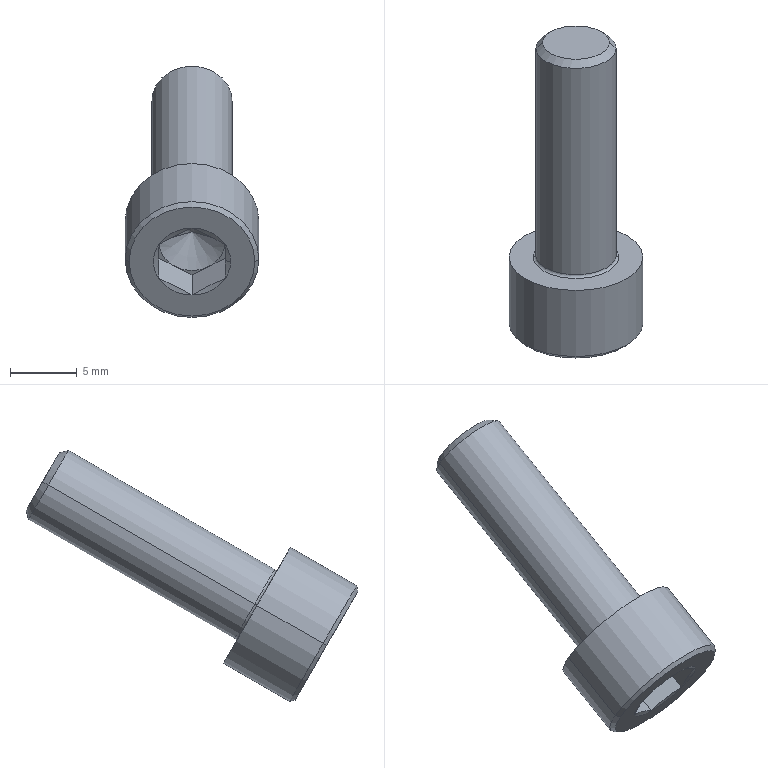Part | SolidWorks | features BaseBody 1 | 1 solid | 34 faces | box 10 x 24.818 x 18.778 mm | volume 916.28 mm3 | plane 15 | cone 13 | cylinder 4 | torus 2 | commonest cylinder face diameters 6 x2 10 x2
STEP:
#1=CARTESIAN_POINT('',(133.,-39.453,-22.778));
#2=VERTEX_POINT('',#1);
#3=CARTESIAN_POINT('',(135.5,-40.703,-23.5));
#4=VERTEX_POINT('',#3);
#5=CARTESIAN_POINT('',(135.5,-40.703,-23.5));
#6=DIRECTION('',(0.866,-0.433,-0.25));
#7=VECTOR('',#6,1000.);
#8=LINE('',#5,#7);
#9=EDGE_CURVE('',#2,#4,#8,.T.);
#10=ORIENTED_EDGE('',*,*,#9,.F.);
#11=CARTESIAN_POINT('',(130.5,-40.703,-23.5));
#12=VERTEX_POINT('',#11);
#13=CARTESIAN_POINT('',(130.5,-40.703,-23.5));
#14=DIRECTION('',(-0.866,-0.433,-0.25));
#15=VECTOR('',#14,1000.);
#16=LINE('',#13,#15);
#17=EDGE_CURVE('',#2,#12,#16,.T.);
#18=ORIENTED_EDGE('',*,*,#17,.T.);
#19=CARTESIAN_POINT('',(131.75,-39.621,-25.375));
#20=VERTEX_POINT('',#19);
#21=CARTESIAN_POINT('',(133.,-40.703,-23.5));
#22=DIRECTION('',(0.,-0.866,-0.5));
#23=DIRECTION('',(1.,0.,0.));
#24=AXIS2_PLACEMENT_3D('',#21,#22,#23);
#25=CIRCLE('',#24,2.5);
#26=EDGE_CURVE('',#12,#20,#25,.T.);
#27=ORIENTED_EDGE('',*,*,#26,.T.);
#28=CARTESIAN_POINT('',(134.25,-39.621,-25.375));
#29=VERTEX_POINT('',#28);
#30=CARTESIAN_POINT('',(133.,-40.703,-23.5));
#31=DIRECTION('',(0.,-0.866,-0.5));
#32=DIRECTION('',(1.,0.,0.));
#33=AXIS2_PLACEMENT_3D('',#30,#31,#32);
#34=CIRCLE('',#33,2.5);
#35=EDGE_CURVE('',#20,#29,#34,.T.);
#36=ORIENTED_EDGE('',*,*,#35,.T.);
#37=CARTESIAN_POINT('',(133.,-40.703,-23.5));
#38=DIRECTION('',(0.,-0.866,-0.5));
#39=DIRECTION('',(1.,0.,0.));
#40=AXIS2_PLACEMENT_3D('',#37,#38,#39);
#41=CIRCLE('',#40,2.5);
#42=EDGE_CURVE('',#29,#4,#41,.T.);
#43=ORIENTED_EDGE('',*,*,#42,.T.);
#44=EDGE_LOOP('',(#10,#18,#27,#36,#43));
#45=FACE_OUTER_BOUND('',#44,.T.);
#46=CARTESIAN_POINT('',(133.,-40.703,-23.5));
#47=DIRECTION('',(0.,-0.866,-0.5));
#48=DIRECTION('',(1.,0.,0.));
#49=AXIS2_PLACEMENT_3D('',#46,#47,#48);
#50=CONICAL_SURFACE('',#49,2.5,1.047);
#51=ADVANCED_FACE('',(#45),#50,.F.);
#52=CARTESIAN_POINT('',(135.5,-43.212,-24.948));
#53=VERTEX_POINT('',#52);
#54=CARTESIAN_POINT('',(135.5,-44.023,-23.75));
#55=VERTEX_POINT('',#54);
#56=CARTESIAN_POINT('',(135.5,-43.212,-24.948));
#57=CARTESIAN_POINT('',(135.5,-43.453,-24.531));
#58=CARTESIAN_POINT('',(135.5,-43.727,-24.134));
#59=CARTESIAN_POINT('',(135.5,-44.023,-23.75));
#60=B_SPLINE_CURVE_WITH_KNOTS('',3,(#56,#57,#58,#59),.UNSPECIFIED.,.F.,.F.,(4,4),(0.003815,0.005271),.UNSPECIFIED.);
#61=EDGE_CURVE('',#53,#55,#60,.T.);
#62=ORIENTED_EDGE('',*,*,#61,.F.);
#63=CARTESIAN_POINT('',(135.887,-43.301,-25.));
#64=VERTEX_POINT('',#63);
#65=CARTESIAN_POINT('',(135.887,-43.301,-25.));
#66=DIRECTION('',(0.9659,-0.2241,-0.1294));
#67=VECTOR('',#66,1000.);
#68=LINE('',#65,#67);
#69=EDGE_CURVE('',#53,#64,#68,.T.);
#70=ORIENTED_EDGE('',*,*,#69,.T.);
#71=CARTESIAN_POINT('',(133.,-43.301,-25.));
#72=DIRECTION('',(0.,-0.866,-0.5));
#73=DIRECTION('',(1.,0.,0.));
#74=AXIS2_PLACEMENT_3D('',#71,#72,#73);
#75=CIRCLE('',#74,2.887);
#76=EDGE_CURVE('',#64,#55,#75,.T.);
#77=ORIENTED_EDGE('',*,*,#76,.T.);
#78=EDGE_LOOP('',(#62,#70,#77));
#79=FACE_OUTER_BOUND('',#78,.T.);
#80=CARTESIAN_POINT('',(133.,-43.301,-25.));
#81=DIRECTION('',(0.,-0.866,-0.5));
#82=DIRECTION('',(1.,0.,0.));
#83=AXIS2_PLACEMENT_3D('',#80,#81,#82);
#84=CONICAL_SURFACE('',#83,2.887,1.309);
#85=ADVANCED_FACE('',(#79),#84,.F.);
#86=CARTESIAN_POINT('',(130.5,-22.084,-12.75));
#87=VERTEX_POINT('',#86);
#88=CARTESIAN_POINT('',(135.5,-22.084,-12.75));
#89=VERTEX_POINT('',#88);
#90=CARTESIAN_POINT('',(133.,-22.084,-12.75));
#91=DIRECTION('',(0.,0.866,0.5));
#92=DIRECTION('',(-1.,0.,0.));
#93=AXIS2_PLACEMENT_3D('',#90,#91,#92);
#94=CIRCLE('',#93,2.5);
#95=EDGE_CURVE('',#87,#89,#94,.T.);
#96=ORIENTED_EDGE('',*,*,#95,.F.);
#97=CARTESIAN_POINT('',(130.,-22.517,-13.));
#98=VERTEX_POINT('',#97);
#99=CARTESIAN_POINT('',(130.5,-22.084,-12.75));
#100=DIRECTION('',(-0.7071,-0.6124,-0.3536));
#101=VECTOR('',#100,1000.);
#102=LINE('',#99,#101);
#103=EDGE_CURVE('',#87,#98,#102,.T.);
#104=ORIENTED_EDGE('',*,*,#103,.T.);
#105=CARTESIAN_POINT('',(136.,-22.517,-13.));
#106=VERTEX_POINT('',#105);
#107=CARTESIAN_POINT('',(133.,-22.517,-13.));
#108=DIRECTION('',(0.,-0.866,-0.5));
#109=DIRECTION('',(-1.,0.,0.));
#110=AXIS2_PLACEMENT_3D('',#107,#108,#109);
#111=CIRCLE('',#110,3.);
#112=EDGE_CURVE('',#106,#98,#111,.T.);
#113=ORIENTED_EDGE('',*,*,#112,.F.);
#114=CARTESIAN_POINT('',(135.5,-22.084,-12.75));
#115=DIRECTION('',(0.7071,-0.6124,-0.3536));
#116=VECTOR('',#115,1000.);
#117=LINE('',#114,#116);
#118=EDGE_CURVE('',#89,#106,#117,.T.);
#119=ORIENTED_EDGE('',*,*,#118,.F.);
#120=EDGE_LOOP('',(#96,#104,#113,#119));
#121=FACE_OUTER_BOUND('',#120,.T.);
#122=CARTESIAN_POINT('',(133.,-22.084,-12.75));
#123=DIRECTION('',(0.,-0.866,-0.5));
#124=DIRECTION('',(1.,0.,0.));
#125=AXIS2_PLACEMENT_3D('',#122,#123,#124);
#126=CONICAL_SURFACE('',#125,2.5,0.7854);
#127=ADVANCED_FACE('',(#121),#126,.T.);
#128=CARTESIAN_POINT('',(136.,-37.932,-21.9));
#129=VERTEX_POINT('',#128);
#130=CARTESIAN_POINT('',(130.,-37.932,-21.9));
#131=VERTEX_POINT('',#130);
#132=CARTESIAN_POINT('',(133.,-37.932,-21.9));
#133=DIRECTION('',(0.,0.866,0.5));
#134=DIRECTION('',(-1.,0.,0.));
#135=AXIS2_PLACEMENT_3D('',#132,#133,#134);
#136=CIRCLE('',#135,3.);
#137=EDGE_CURVE('',#129,#131,#136,.T.);
#138=ORIENTED_EDGE('',*,*,#137,.F.);
#139=CARTESIAN_POINT('',(136.2,-38.105,-22.));
#140=VERTEX_POINT('',#139);
#141=CARTESIAN_POINT('',(136.2,-37.932,-21.9));
#142=DIRECTION('',(0.,-0.5,0.866));
#143=DIRECTION('',(0.,-0.866,-0.5));
#144=AXIS2_PLACEMENT_3D('',#141,#142,#143);
#145=CIRCLE('',#144,0.2);
#146=EDGE_CURVE('',#129,#140,#145,.T.);
#147=ORIENTED_EDGE('',*,*,#146,.T.);
#148=CARTESIAN_POINT('',(129.8,-38.105,-22.));
#149=VERTEX_POINT('',#148);
#150=CARTESIAN_POINT('',(133.,-38.105,-22.));
#151=DIRECTION('',(0.,-0.866,-0.5));
#152=DIRECTION('',(-1.,0.,0.));
#153=AXIS2_PLACEMENT_3D('',#150,#151,#152);
#154=CIRCLE('',#153,3.2);
#155=EDGE_CURVE('',#149,#140,#154,.T.);
#156=ORIENTED_EDGE('',*,*,#155,.F.);
#157=CARTESIAN_POINT('',(129.8,-37.932,-21.9));
#158=DIRECTION('',(0.,0.5,-0.866));
#159=DIRECTION('',(0.,0.866,0.5));
#160=AXIS2_PLACEMENT_3D('',#157,#158,#159);
#161=CIRCLE('',#160,0.2);
#162=EDGE_CURVE('',#131,#149,#161,.T.);
#163=ORIENTED_EDGE('',*,*,#162,.F.);
#164=EDGE_LOOP('',(#138,#147,#156,#163));
#165=FACE_OUTER_BOUND('',#164,.T.);
#166=CARTESIAN_POINT('',(133.,-37.932,-21.9));
#167=DIRECTION('',(0.,0.866,0.5));
#168=DIRECTION('',(-1.,0.,0.));
#169=AXIS2_PLACEMENT_3D('',#166,#167,#168);
#170=TOROIDAL_SURFACE('',#169,3.2,0.2);
#171=ADVANCED_FACE('',(#165),#170,.F.);
#172=ORIENTED_EDGE('',*,*,#112,.T.);
#173=CARTESIAN_POINT('',(130.,-22.084,-12.75));
#174=DIRECTION('',(0.,-0.866,-0.5));
#175=VECTOR('',#174,1000.);
#176=LINE('',#173,#175);
#177=EDGE_CURVE('',#98,#131,#176,.T.);
#178=ORIENTED_EDGE('',*,*,#177,.T.);
#179=CARTESIAN_POINT('',(133.,-37.932,-21.9));
#180=DIRECTION('',(0.,0.866,0.5));
#181=DIRECTION('',(-1.,0.,0.));
#182=AXIS2_PLACEMENT_3D('',#179,#180,#181);
#183=CIRCLE('',#182,3.);
#184=EDGE_CURVE('',#131,#129,#183,.T.);
#185=ORIENTED_EDGE('',*,*,#184,.T.);
#186=CARTESIAN_POINT('',(136.,-22.084,-12.75));
#187=DIRECTION('',(0.,-0.866,-0.5));
#188=VECTOR('',#187,1000.);
#189=LINE('',#186,#188);
#190=EDGE_CURVE('',#106,#129,#189,.T.);
#191=ORIENTED_EDGE('',*,*,#190,.F.);
#192=EDGE_LOOP('',(#172,#178,#185,#191));
#193=FACE_OUTER_BOUND('',#192,.T.);
#194=CARTESIAN_POINT('',(133.,-22.084,-12.75));
#195=DIRECTION('',(0.,-0.866,-0.5));
#196=DIRECTION('',(1.,0.,0.));
#197=AXIS2_PLACEMENT_3D('',#194,#195,#196);
#198=CYLINDRICAL_SURFACE('',#197,3.);
#199=ADVANCED_FACE('',(#193),#198,.T.);
#200=CARTESIAN_POINT('',(137.7,-43.301,-25.));
#201=VERTEX_POINT('',#200);
#202=CARTESIAN_POINT('',(128.3,-43.301,-25.));
#203=VERTEX_POINT('',#202);
#204=CARTESIAN_POINT('',(133.,-43.301,-25.));
#205=DIRECTION('',(0.,-0.866,-0.5));
#206=DIRECTION('',(-1.,0.,0.));
#207=AXIS2_PLACEMENT_3D('',#204,#205,#206);
#208=CIRCLE('',#207,4.7);
#209=EDGE_CURVE('',#201,#203,#208,.T.);
#210=ORIENTED_EDGE('',*,*,#209,.F.);
#211=CARTESIAN_POINT('',(138.,-43.041,-24.85));
#212=VERTEX_POINT('',#211);
#213=CARTESIAN_POINT('',(138.,-43.041,-24.85));
#214=DIRECTION('',(0.7071,0.6124,0.3536));
#215=VECTOR('',#214,1000.);
#216=LINE('',#213,#215);
#217=EDGE_CURVE('',#201,#212,#216,.T.);
#218=ORIENTED_EDGE('',*,*,#217,.T.);
#219=CARTESIAN_POINT('',(128.,-43.041,-24.85));
#220=VERTEX_POINT('',#219);
#221=CARTESIAN_POINT('',(133.,-43.041,-24.85));
#222=DIRECTION('',(0.,0.866,0.5));
#223=DIRECTION('',(-1.,0.,0.));
#224=AXIS2_PLACEMENT_3D('',#221,#222,#223);
#225=CIRCLE('',#224,5.);
#226=EDGE_CURVE('',#220,#212,#225,.T.);
#227=ORIENTED_EDGE('',*,*,#226,.F.);
#228=CARTESIAN_POINT('',(128.,-43.041,-24.85));
#229=DIRECTION('',(-0.7071,0.6124,0.3536));
#230=VECTOR('',#229,1000.);
#231=LINE('',#228,#230);
#232=EDGE_CURVE('',#203,#220,#231,.T.);
#233=ORIENTED_EDGE('',*,*,#232,.F.);
#234=EDGE_LOOP('',(#210,#218,#227,#233));
#235=FACE_OUTER_BOUND('',#234,.T.);
#236=CARTESIAN_POINT('',(133.,-43.041,-24.85));
#237=DIRECTION('',(0.,0.866,0.5));
#238=DIRECTION('',(-1.,0.,0.));
#239=AXIS2_PLACEMENT_3D('',#236,#237,#238);
#240=CONICAL_SURFACE('',#239,5.,0.7854);
#241=ADVANCED_FACE('',(#235),#240,.T.);
#242=CARTESIAN_POINT('',(128.,-38.105,-22.));
#243=VERTEX_POINT('',#242);
#244=CARTESIAN_POINT('',(138.,-38.105,-22.));
#245=VERTEX_POINT('',#244);
#246=CARTESIAN_POINT('',(133.,-38.105,-22.));
#247=DIRECTION('',(0.,0.866,0.5));
#248=DIRECTION('',(-1.,0.,0.));
#249=AXIS2_PLACEMENT_3D('',#246,#247,#248);
#250=CIRCLE('',#249,5.);
#251=EDGE_CURVE('',#243,#245,#250,.T.);
#252=ORIENTED_EDGE('',*,*,#251,.F.);
#253=CARTESIAN_POINT('',(128.,-38.105,-22.));
#254=DIRECTION('',(0.,-0.866,-0.5));
#255=VECTOR('',#254,1000.);
#256=LINE('',#253,#255);
#257=EDGE_CURVE('',#243,#220,#256,.T.);
#258=ORIENTED_EDGE('',*,*,#257,.T.);
#259=ORIENTED_EDGE('',*,*,#226,.T.);
#260=CARTESIAN_POINT('',(138.,-38.105,-22.));
#261=DIRECTION('',(0.,-0.866,-0.5));
#262=VECTOR('',#261,1000.);
#263=LINE('',#260,#262);
#264=EDGE_CURVE('',#245,#212,#263,.T.);
#265=ORIENTED_EDGE('',*,*,#264,.F.);
#266=EDGE_LOOP('',(#252,#258,#259,#265));
#267=FACE_OUTER_BOUND('',#266,.T.);
#268=CARTESIAN_POINT('',(133.,-38.105,-22.));
#269=DIRECTION('',(0.,-0.866,-0.5));
#270=DIRECTION('',(1.,0.,0.));
#271=AXIS2_PLACEMENT_3D('',#268,#269,#270);
#272=CYLINDRICAL_SURFACE('',#271,5.);
#273=ADVANCED_FACE('',(#267),#272,.T.);
#274=ORIENTED_EDGE('',*,*,#155,.T.);
#275=CARTESIAN_POINT('',(133.,-38.105,-22.));
#276=DIRECTION('',(0.,-0.866,-0.5));
#277=DIRECTION('',(-1.,0.,0.));
#278=AXIS2_PLACEMENT_3D('',#275,#276,#277);
#279=CIRCLE('',#278,3.2);
#280=EDGE_CURVE('',#140,#149,#279,.T.);
#281=ORIENTED_EDGE('',*,*,#280,.T.);
#282=EDGE_LOOP('',(#274,#281));
#283=FACE_BOUND('',#282,.T.);
#284=CARTESIAN_POINT('',(133.,-38.105,-22.));
#285=DIRECTION('',(0.,0.866,0.5));
#286=DIRECTION('',(-1.,0.,0.));
#287=AXIS2_PLACEMENT_3D('',#284,#285,#286);
#288=CIRCLE('',#287,5.);
#289=EDGE_CURVE('',#245,#243,#288,.T.);
#290=ORIENTED_EDGE('',*,*,#289,.T.);
#291=ORIENTED_EDGE('',*,*,#251,.T.);
#292=EDGE_LOOP('',(#290,#291));
#293=FACE_OUTER_BOUND('',#292,.T.);
#294=CARTESIAN_POINT('',(133.,-38.105,-22.));
#295=DIRECTION('',(0.,0.866,0.5));
#296=DIRECTION('',(-1.,0.,0.));
#297=AXIS2_PLACEMENT_3D('',#294,#295,#296);
#298=PLANE('',#297);
#299=ADVANCED_FACE('',(#283,#293),#298,.T.);
#300=ORIENTED_EDGE('',*,*,#257,.F.);
#301=ORIENTED_EDGE('',*,*,#289,.F.);
#302=ORIENTED_EDGE('',*,*,#264,.T.);
#303=CARTESIAN_POINT('',(133.,-43.041,-24.85));
#304=DIRECTION('',(0.,0.866,0.5));
#305=DIRECTION('',(-1.,0.,0.));
#306=AXIS2_PLACEMENT_3D('',#303,#304,#305);
#307=CIRCLE('',#306,5.);
#308=EDGE_CURVE('',#212,#220,#307,.T.);
#309=ORIENTED_EDGE('',*,*,#308,.T.);
#310=EDGE_LOOP('',(#300,#301,#302,#309));
#311=FACE_OUTER_BOUND('',#310,.T.);
#312=CARTESIAN_POINT('',(133.,-38.105,-22.));
#313=DIRECTION('',(0.,-0.866,-0.5));
#314=DIRECTION('',(1.,0.,0.));
#315=AXIS2_PLACEMENT_3D('',#312,#313,#314);
#316=CYLINDRICAL_SURFACE('',#315,5.);
#317=ADVANCED_FACE('',(#311),#316,.T.);
#318=CARTESIAN_POINT('',(130.5,-44.023,-23.75));
#319=VERTEX_POINT('',#318);
#320=CARTESIAN_POINT('',(130.5,-42.58,-26.25));
#321=VERTEX_POINT('',#320);
#322=CARTESIAN_POINT('',(133.,-43.301,-25.));
#323=DIRECTION('',(0.,-0.866,-0.5));
#324=DIRECTION('',(1.,0.,0.));
#325=AXIS2_PLACEMENT_3D('',#322,#323,#324);
#326=CIRCLE('',#325,2.887);
#327=EDGE_CURVE('',#319,#321,#326,.T.);
#328=ORIENTED_EDGE('',*,*,#327,.F.);
#329=CARTESIAN_POINT('',(133.,-44.745,-22.5));
#330=VERTEX_POINT('',#329);
#331=CARTESIAN_POINT('',(133.,-43.301,-25.));
#332=DIRECTION('',(0.,-0.866,-0.5));
#333=DIRECTION('',(1.,0.,0.));
#334=AXIS2_PLACEMENT_3D('',#331,#332,#333);
#335=CIRCLE('',#334,2.887);
#336=EDGE_CURVE('',#330,#319,#335,.T.);
#337=ORIENTED_EDGE('',*,*,#336,.F.);
#338=CARTESIAN_POINT('',(133.,-43.301,-25.));
#339=DIRECTION('',(0.,-0.866,-0.5));
#340=DIRECTION('',(1.,0.,0.));
#341=AXIS2_PLACEMENT_3D('',#338,#339,#340);
#342=CIRCLE('',#341,2.887);
#343=EDGE_CURVE('',#55,#330,#342,.T.);
#344=ORIENTED_EDGE('',*,*,#343,.F.);
#345=ORIENTED_EDGE('',*,*,#76,.F.);
#346=CARTESIAN_POINT('',(135.5,-42.58,-26.25));
#347=VERTEX_POINT('',#346);
#348=CARTESIAN_POINT('',(133.,-43.301,-25.));
#349=DIRECTION('',(0.,-0.866,-0.5));
#350=DIRECTION('',(1.,0.,0.));
#351=AXIS2_PLACEMENT_3D('',#348,#349,#350);
#352=CIRCLE('',#351,2.887);
#353=EDGE_CURVE('',#347,#64,#352,.T.);
#354=ORIENTED_EDGE('',*,*,#353,.F.);
#355=CARTESIAN_POINT('',(133.,-41.858,-27.5));
#356=VERTEX_POINT('',#355);
#357=CARTESIAN_POINT('',(133.,-43.301,-25.));
#358=DIRECTION('',(0.,-0.866,-0.5));
#359=DIRECTION('',(1.,0.,0.));
#360=AXIS2_PLACEMENT_3D('',#357,#358,#359);
#361=CIRCLE('',#360,2.887);
#362=EDGE_CURVE('',#356,#347,#361,.T.);
#363=ORIENTED_EDGE('',*,*,#362,.F.);
#364=CARTESIAN_POINT('',(133.,-43.301,-25.));
#365=DIRECTION('',(0.,-0.866,-0.5));
#366=DIRECTION('',(1.,0.,0.));
#367=AXIS2_PLACEMENT_3D('',#364,#365,#366);
#368=CIRCLE('',#367,2.887);
#369=EDGE_CURVE('',#321,#356,#368,.T.);
#370=ORIENTED_EDGE('',*,*,#369,.F.);
#371=EDGE_LOOP('',(#328,#337,#344,#345,#354,#363,#370));
#372=FACE_BOUND('',#371,.T.);
#373=CARTESIAN_POINT('',(133.,-43.301,-25.));
#374=DIRECTION('',(0.,-0.866,-0.5));
#375=DIRECTION('',(-1.,0.,0.));
#376=AXIS2_PLACEMENT_3D('',#373,#374,#375);
#377=CIRCLE('',#376,4.7);
#378=EDGE_CURVE('',#203,#201,#377,.T.);
#379=ORIENTED_EDGE('',*,*,#378,.T.);
#380=ORIENTED_EDGE('',*,*,#209,.T.);
#381=EDGE_LOOP('',(#379,#380));
#382=FACE_OUTER_BOUND('',#381,.T.);
#383=CARTESIAN_POINT('',(133.,-43.301,-25.));
#384=DIRECTION('',(0.,0.866,0.5));
#385=DIRECTION('',(-1.,0.,0.));
#386=AXIS2_PLACEMENT_3D('',#383,#384,#385);
#387=PLANE('',#386);
#388=ADVANCED_FACE('',(#372,#382),#387,.F.);
#389=ORIENTED_EDGE('',*,*,#217,.F.);
#390=ORIENTED_EDGE('',*,*,#378,.F.);
#391=ORIENTED_EDGE('',*,*,#232,.T.);
#392=ORIENTED_EDGE('',*,*,#308,.F.);
#393=EDGE_LOOP('',(#389,#390,#391,#392));
#394=FACE_OUTER_BOUND('',#393,.T.);
#395=CARTESIAN_POINT('',(133.,-43.041,-24.85));
#396=DIRECTION('',(0.,0.866,0.5));
#397=DIRECTION('',(-1.,0.,0.));
#398=AXIS2_PLACEMENT_3D('',#395,#396,#397);
#399=CONICAL_SURFACE('',#398,5.,0.7854);
#400=ADVANCED_FACE('',(#394),#399,.T.);
#401=ORIENTED_EDGE('',*,*,#177,.F.);
#402=CARTESIAN_POINT('',(133.,-22.517,-13.));
#403=DIRECTION('',(0.,-0.866,-0.5));
#404=DIRECTION('',(-1.,0.,0.));
#405=AXIS2_PLACEMENT_3D('',#402,#403,#404);
#406=CIRCLE('',#405,3.);
#407=EDGE_CURVE('',#98,#106,#406,.T.);
#408=ORIENTED_EDGE('',*,*,#407,.T.);
#409=ORIENTED_EDGE('',*,*,#190,.T.);
#410=ORIENTED_EDGE('',*,*,#137,.T.);
#411=EDGE_LOOP('',(#401,#408,#409,#410));
#412=FACE_OUTER_BOUND('',#411,.T.);
#413=CARTESIAN_POINT('',(133.,-22.084,-12.75));
#414=DIRECTION('',(0.,-0.866,-0.5));
#415=DIRECTION('',(1.,0.,0.));
#416=AXIS2_PLACEMENT_3D('',#413,#414,#415);
#417=CYLINDRICAL_SURFACE('',#416,3.);
#418=ADVANCED_FACE('',(#412),#417,.T.);
#419=CARTESIAN_POINT('',(133.,-22.084,-12.75));
#420=DIRECTION('',(0.,0.866,0.5));
#421=DIRECTION('',(-1.,0.,0.));
#422=AXIS2_PLACEMENT_3D('',#419,#420,#421);
#423=CIRCLE('',#422,2.5);
#424=EDGE_CURVE('',#89,#87,#423,.T.);
#425=ORIENTED_EDGE('',*,*,#424,.T.);
#426=ORIENTED_EDGE('',*,*,#95,.T.);
#427=EDGE_LOOP('',(#425,#426));
#428=FACE_OUTER_BOUND('',#427,.T.);
#429=CARTESIAN_POINT('',(133.,-22.084,-12.75));
#430=DIRECTION('',(0.,0.866,0.5));
#431=DIRECTION('',(-1.,0.,0.));
#432=AXIS2_PLACEMENT_3D('',#429,#430,#431);
#433=PLANE('',#432);
#434=ADVANCED_FACE('',(#428),#433,.T.);
#435=ORIENTED_EDGE('',*,*,#146,.F.);
#436=ORIENTED_EDGE('',*,*,#184,.F.);
#437=ORIENTED_EDGE('',*,*,#162,.T.);
#438=ORIENTED_EDGE('',*,*,#280,.F.);
#439=EDGE_LOOP('',(#435,#436,#437,#438));
#440=FACE_OUTER_BOUND('',#439,.T.);
#441=CARTESIAN_POINT('',(133.,-37.932,-21.9));
#442=DIRECTION('',(0.,0.866,0.5));
#443=DIRECTION('',(-1.,0.,0.));
#444=AXIS2_PLACEMENT_3D('',#441,#442,#443);
#445=TOROIDAL_SURFACE('',#444,3.2,0.2);
#446=ADVANCED_FACE('',(#440),#445,.F.);
#447=ORIENTED_EDGE('',*,*,#103,.F.);
#448=ORIENTED_EDGE('',*,*,#424,.F.);
#449=ORIENTED_EDGE('',*,*,#118,.T.);
#450=ORIENTED_EDGE('',*,*,#407,.F.);
#451=EDGE_LOOP('',(#447,#448,#449,#450));
#452=FACE_OUTER_BOUND('',#451,.T.);
#453=CARTESIAN_POINT('',(133.,-22.084,-12.75));
#454=DIRECTION('',(0.,-0.866,-0.5));
#455=DIRECTION('',(1.,0.,0.));
#456=AXIS2_PLACEMENT_3D('',#453,#454,#455);
#457=CONICAL_SURFACE('',#456,2.5,0.7854);
#458=ADVANCED_FACE('',(#452),#457,.T.);
#459=ORIENTED_EDGE('',*,*,#336,.T.);
#460=CARTESIAN_POINT('',(133.,-44.745,-22.5));
#461=CARTESIAN_POINT('',(132.583,-44.569,-22.676));
#462=CARTESIAN_POINT('',(131.75,-44.26,-23.054));
#463=CARTESIAN_POINT('',(130.917,-44.087,-23.509));
#464=CARTESIAN_POINT('',(130.5,-44.023,-23.75));
#465=B_SPLINE_CURVE_WITH_KNOTS('',3,(#460,#461,#462,#463,#464),.UNSPECIFIED.,.F.,.F.,(4,1,4),(0.000000231,0.001444,0.002887),.UNSPECIFIED.);
#466=EDGE_CURVE('',#330,#319,#465,.T.);
#467=ORIENTED_EDGE('',*,*,#466,.F.);
#468=EDGE_LOOP('',(#459,#467));
#469=FACE_OUTER_BOUND('',#468,.T.);
#470=CARTESIAN_POINT('',(133.,-43.301,-25.));
#471=DIRECTION('',(0.,-0.866,-0.5));
#472=DIRECTION('',(1.,0.,0.));
#473=AXIS2_PLACEMENT_3D('',#470,#471,#472);
#474=CONICAL_SURFACE('',#473,2.887,1.309);
#475=ADVANCED_FACE('',(#469),#474,.F.);
#476=ORIENTED_EDGE('',*,*,#327,.T.);
#477=CARTESIAN_POINT('',(130.5,-44.023,-23.75));
#478=CARTESIAN_POINT('',(130.5,-43.728,-24.133));
#479=CARTESIAN_POINT('',(130.5,-43.454,-24.529));
#480=CARTESIAN_POINT('',(130.5,-42.972,-25.363));
#481=CARTESIAN_POINT('',(130.5,-42.764,-25.802));
#482=CARTESIAN_POINT('',(130.5,-42.58,-26.25));
#483=B_SPLINE_CURVE_WITH_KNOTS('',3,(#477,#478,#479,#480,#481,#482),.UNSPECIFIED.,.F.,.F.,(4,2,4),(0.0002925,0.001736,0.003179),.UNSPECIFIED.);
#484=EDGE_CURVE('',#319,#321,#483,.T.);
#485=ORIENTED_EDGE('',*,*,#484,.F.);
#486=EDGE_LOOP('',(#476,#485));
#487=FACE_OUTER_BOUND('',#486,.T.);
#488=CARTESIAN_POINT('',(133.,-43.301,-25.));
#489=DIRECTION('',(0.,-0.866,-0.5));
#490=DIRECTION('',(1.,0.,0.));
#491=AXIS2_PLACEMENT_3D('',#488,#489,#490);
#492=CONICAL_SURFACE('',#491,2.887,1.309);
#493=ADVANCED_FACE('',(#487),#492,.F.);
#494=ORIENTED_EDGE('',*,*,#369,.T.);
#495=CARTESIAN_POINT('',(130.5,-42.58,-26.25));
#496=CARTESIAN_POINT('',(130.917,-42.403,-26.426));
#497=CARTESIAN_POINT('',(131.75,-42.095,-26.804));
#498=CARTESIAN_POINT('',(132.583,-41.922,-27.259));
#499=CARTESIAN_POINT('',(133.,-41.858,-27.5));
#500=B_SPLINE_CURVE_WITH_KNOTS('',3,(#495,#496,#497,#498,#499),.UNSPECIFIED.,.F.,.F.,(4,1,4),(0.000000231,0.001444,0.002887),.UNSPECIFIED.);
#501=EDGE_CURVE('',#321,#356,#500,.T.);
#502=ORIENTED_EDGE('',*,*,#501,.F.);
#503=EDGE_LOOP('',(#494,#502));
#504=FACE_OUTER_BOUND('',#503,.T.);
#505=CARTESIAN_POINT('',(133.,-43.301,-25.));
#506=DIRECTION('',(0.,-0.866,-0.5));
#507=DIRECTION('',(1.,0.,0.));
#508=AXIS2_PLACEMENT_3D('',#505,#506,#507);
#509=CONICAL_SURFACE('',#508,2.887,1.309);
#510=ADVANCED_FACE('',(#504),#509,.F.);
#511=ORIENTED_EDGE('',*,*,#362,.T.);
#512=CARTESIAN_POINT('',(133.,-41.858,-27.5));
#513=CARTESIAN_POINT('',(133.417,-41.922,-27.259));
#514=CARTESIAN_POINT('',(134.25,-42.095,-26.804));
#515=CARTESIAN_POINT('',(135.083,-42.403,-26.426));
#516=CARTESIAN_POINT('',(135.5,-42.58,-26.25));
#517=B_SPLINE_CURVE_WITH_KNOTS('',3,(#512,#513,#514,#515,#516),.UNSPECIFIED.,.F.,.F.,(4,1,4),(0.000000231,0.001444,0.002887),.UNSPECIFIED.);
#518=EDGE_CURVE('',#356,#347,#517,.T.);
#519=ORIENTED_EDGE('',*,*,#518,.F.);
#520=EDGE_LOOP('',(#511,#519));
#521=FACE_OUTER_BOUND('',#520,.T.);
#522=CARTESIAN_POINT('',(133.,-43.301,-25.));
#523=DIRECTION('',(0.,-0.866,-0.5));
#524=DIRECTION('',(1.,0.,0.));
#525=AXIS2_PLACEMENT_3D('',#522,#523,#524);
#526=CONICAL_SURFACE('',#525,2.887,1.309);
#527=ADVANCED_FACE('',(#521),#526,.F.);
#528=ORIENTED_EDGE('',*,*,#69,.F.);
#529=CARTESIAN_POINT('',(135.5,-42.58,-26.25));
#530=CARTESIAN_POINT('',(135.5,-42.764,-25.803));
#531=CARTESIAN_POINT('',(135.5,-42.971,-25.364));
#532=CARTESIAN_POINT('',(135.5,-43.212,-24.948));
#533=B_SPLINE_CURVE_WITH_KNOTS('',3,(#529,#530,#531,#532),.UNSPECIFIED.,.F.,.F.,(4,4),(0.002365,0.003815),.UNSPECIFIED.);
#534=EDGE_CURVE('',#347,#53,#533,.T.);
#535=ORIENTED_EDGE('',*,*,#534,.F.);
#536=ORIENTED_EDGE('',*,*,#353,.T.);
#537=EDGE_LOOP('',(#528,#535,#536));
#538=FACE_OUTER_BOUND('',#537,.T.);
#539=CARTESIAN_POINT('',(133.,-43.301,-25.));
#540=DIRECTION('',(0.,-0.866,-0.5));
#541=DIRECTION('',(1.,0.,0.));
#542=AXIS2_PLACEMENT_3D('',#539,#540,#541);
#543=CONICAL_SURFACE('',#542,2.887,1.309);
#544=ADVANCED_FACE('',(#538),#543,.F.);
#545=ORIENTED_EDGE('',*,*,#343,.T.);
#546=CARTESIAN_POINT('',(135.5,-44.023,-23.75));
#547=CARTESIAN_POINT('',(135.083,-44.087,-23.509));
#548=CARTESIAN_POINT('',(134.25,-44.26,-23.054));
#549=CARTESIAN_POINT('',(133.417,-44.569,-22.676));
#550=CARTESIAN_POINT('',(133.,-44.745,-22.5));
#551=B_SPLINE_CURVE_WITH_KNOTS('',3,(#546,#547,#548,#549,#550),.UNSPECIFIED.,.F.,.F.,(4,1,4),(0.000000231,0.001444,0.002887),.UNSPECIFIED.);
#552=EDGE_CURVE('',#55,#330,#551,.T.);
#553=ORIENTED_EDGE('',*,*,#552,.F.);
#554=EDGE_LOOP('',(#545,#553));
#555=FACE_OUTER_BOUND('',#554,.T.);
#556=CARTESIAN_POINT('',(133.,-43.301,-25.));
#557=DIRECTION('',(0.,-0.866,-0.5));
#558=DIRECTION('',(1.,0.,0.));
#559=AXIS2_PLACEMENT_3D('',#556,#557,#558);
#560=CONICAL_SURFACE('',#559,2.887,1.309);
#561=ADVANCED_FACE('',(#555),#560,.F.);
#562=ORIENTED_EDGE('',*,*,#17,.F.);
#563=ORIENTED_EDGE('',*,*,#9,.T.);
#564=CARTESIAN_POINT('',(134.25,-41.786,-21.625));
#565=VERTEX_POINT('',#564);
#566=CARTESIAN_POINT('',(133.,-40.703,-23.5));
#567=DIRECTION('',(0.,-0.866,-0.5));
#568=DIRECTION('',(1.,0.,0.));
#569=AXIS2_PLACEMENT_3D('',#566,#567,#568);
#570=CIRCLE('',#569,2.5);
#571=EDGE_CURVE('',#4,#565,#570,.T.);
#572=ORIENTED_EDGE('',*,*,#571,.T.);
#573=CARTESIAN_POINT('',(131.75,-41.786,-21.625));
#574=VERTEX_POINT('',#573);
#575=CARTESIAN_POINT('',(133.,-40.703,-23.5));
#576=DIRECTION('',(0.,-0.866,-0.5));
#577=DIRECTION('',(1.,0.,0.));
#578=AXIS2_PLACEMENT_3D('',#575,#576,#577);
#579=CIRCLE('',#578,2.5);
#580=EDGE_CURVE('',#565,#574,#579,.T.);
#581=ORIENTED_EDGE('',*,*,#580,.T.);
#582=CARTESIAN_POINT('',(133.,-40.703,-23.5));
#583=DIRECTION('',(0.,-0.866,-0.5));
#584=DIRECTION('',(1.,0.,0.));
#585=AXIS2_PLACEMENT_3D('',#582,#583,#584);
#586=CIRCLE('',#585,2.5);
#587=EDGE_CURVE('',#574,#12,#586,.T.);
#588=ORIENTED_EDGE('',*,*,#587,.T.);
#589=EDGE_LOOP('',(#562,#563,#572,#581,#588));
#590=FACE_OUTER_BOUND('',#589,.T.);
#591=CARTESIAN_POINT('',(133.,-40.703,-23.5));
#592=DIRECTION('',(0.,-0.866,-0.5));
#593=DIRECTION('',(1.,0.,0.));
#594=AXIS2_PLACEMENT_3D('',#591,#592,#593);
#595=CONICAL_SURFACE('',#594,2.5,1.047);
#596=ADVANCED_FACE('',(#590),#595,.F.);
#597=ORIENTED_EDGE('',*,*,#571,.F.);
#598=CARTESIAN_POINT('',(135.5,-41.425,-22.25));
#599=VERTEX_POINT('',#598);
#600=CARTESIAN_POINT('',(135.5,-39.982,-24.75));
#601=DIRECTION('',(0.,-0.5,0.866));
#602=VECTOR('',#601,1000.);
#603=LINE('',#600,#602);
#604=EDGE_CURVE('',#4,#599,#603,.T.);
#605=ORIENTED_EDGE('',*,*,#604,.T.);
#606=CARTESIAN_POINT('',(135.5,-41.425,-22.25));
#607=DIRECTION('',(-0.866,-0.25,0.433));
#608=VECTOR('',#607,1000.);
#609=LINE('',#606,#608);
#610=EDGE_CURVE('',#599,#565,#609,.T.);
#611=ORIENTED_EDGE('',*,*,#610,.T.);
#612=EDGE_LOOP('',(#597,#605,#611));
#613=FACE_OUTER_BOUND('',#612,.T.);
#614=CARTESIAN_POINT('',(133.,-42.147,-21.));
#615=DIRECTION('',(0.,-0.866,-0.5));
#616=DIRECTION('',(1.,0.,0.));
#617=AXIS2_PLACEMENT_3D('',#614,#615,#616);
#618=PLANE('',#617);
#619=ADVANCED_FACE('',(#613),#618,.T.);
#620=ORIENTED_EDGE('',*,*,#42,.F.);
#621=CARTESIAN_POINT('',(135.5,-39.982,-24.75));
#622=VERTEX_POINT('',#621);
#623=CARTESIAN_POINT('',(133.,-39.26,-26.));
#624=DIRECTION('',(0.866,-0.25,0.433));
#625=VECTOR('',#624,1000.);
#626=LINE('',#623,#625);
#627=EDGE_CURVE('',#29,#622,#626,.T.);
#628=ORIENTED_EDGE('',*,*,#627,.T.);
#629=CARTESIAN_POINT('',(135.5,-39.982,-24.75));
#630=DIRECTION('',(0.,-0.5,0.866));
#631=VECTOR('',#630,1000.);
#632=LINE('',#629,#631);
#633=EDGE_CURVE('',#622,#4,#632,.T.);
#634=ORIENTED_EDGE('',*,*,#633,.T.);
#635=EDGE_LOOP('',(#620,#628,#634));
#636=FACE_OUTER_BOUND('',#635,.T.);
#637=CARTESIAN_POINT('',(133.,-42.147,-21.));
#638=DIRECTION('',(0.,-0.866,-0.5));
#639=DIRECTION('',(1.,0.,0.));
#640=AXIS2_PLACEMENT_3D('',#637,#638,#639);
#641=PLANE('',#640);
#642=ADVANCED_FACE('',(#636),#641,.T.);
#643=ORIENTED_EDGE('',*,*,#35,.F.);
#644=CARTESIAN_POINT('',(133.,-39.26,-26.));
#645=VERTEX_POINT('',#644);
#646=CARTESIAN_POINT('',(130.5,-39.982,-24.75));
#647=DIRECTION('',(0.866,0.25,-0.433));
#648=VECTOR('',#647,1000.);
#649=LINE('',#646,#648);
#650=EDGE_CURVE('',#20,#645,#649,.T.);
#651=ORIENTED_EDGE('',*,*,#650,.T.);
#652=CARTESIAN_POINT('',(133.,-39.26,-26.));
#653=DIRECTION('',(0.866,-0.25,0.433));
#654=VECTOR('',#653,1000.);
#655=LINE('',#652,#654);
#656=EDGE_CURVE('',#645,#29,#655,.T.);
#657=ORIENTED_EDGE('',*,*,#656,.T.);
#658=EDGE_LOOP('',(#643,#651,#657));
#659=FACE_OUTER_BOUND('',#658,.T.);
#660=CARTESIAN_POINT('',(133.,-42.147,-21.));
#661=DIRECTION('',(0.,-0.866,-0.5));
#662=DIRECTION('',(1.,0.,0.));
#663=AXIS2_PLACEMENT_3D('',#660,#661,#662);
#664=PLANE('',#663);
#665=ADVANCED_FACE('',(#659),#664,.T.);
#666=ORIENTED_EDGE('',*,*,#26,.F.);
#667=CARTESIAN_POINT('',(130.5,-39.982,-24.75));
#668=VERTEX_POINT('',#667);
#669=CARTESIAN_POINT('',(130.5,-41.425,-22.25));
#670=DIRECTION('',(0.,0.5,-0.866));
#671=VECTOR('',#670,1000.);
#672=LINE('',#669,#671);
#673=EDGE_CURVE('',#12,#668,#672,.T.);
#674=ORIENTED_EDGE('',*,*,#673,.T.);
#675=CARTESIAN_POINT('',(130.5,-39.982,-24.75));
#676=DIRECTION('',(0.866,0.25,-0.433));
#677=VECTOR('',#676,1000.);
#678=LINE('',#675,#677);
#679=EDGE_CURVE('',#668,#20,#678,.T.);
#680=ORIENTED_EDGE('',*,*,#679,.T.);
#681=EDGE_LOOP('',(#666,#674,#680));
#682=FACE_OUTER_BOUND('',#681,.T.);
#683=CARTESIAN_POINT('',(133.,-42.147,-21.));
#684=DIRECTION('',(0.,-0.866,-0.5));
#685=DIRECTION('',(1.,0.,0.));
#686=AXIS2_PLACEMENT_3D('',#683,#684,#685);
#687=PLANE('',#686);
#688=ADVANCED_FACE('',(#682),#687,.T.);
#689=ORIENTED_EDGE('',*,*,#580,.F.);
#690=CARTESIAN_POINT('',(133.,-42.147,-21.));
#691=VERTEX_POINT('',#690);
#692=CARTESIAN_POINT('',(135.5,-41.425,-22.25));
#693=DIRECTION('',(-0.866,-0.25,0.433));
#694=VECTOR('',#693,1000.);
#695=LINE('',#692,#694);
#696=EDGE_CURVE('',#565,#691,#695,.T.);
#697=ORIENTED_EDGE('',*,*,#696,.T.);
#698=CARTESIAN_POINT('',(133.,-42.147,-21.));
#699=DIRECTION('',(-0.866,0.25,-0.433));
#700=VECTOR('',#699,1000.);
#701=LINE('',#698,#700);
#702=EDGE_CURVE('',#691,#574,#701,.T.);
#703=ORIENTED_EDGE('',*,*,#702,.T.);
#704=EDGE_LOOP('',(#689,#697,#703));
#705=FACE_OUTER_BOUND('',#704,.T.);
#706=CARTESIAN_POINT('',(133.,-42.147,-21.));
#707=DIRECTION('',(0.,-0.866,-0.5));
#708=DIRECTION('',(1.,0.,0.));
#709=AXIS2_PLACEMENT_3D('',#706,#707,#708);
#710=PLANE('',#709);
#711=ADVANCED_FACE('',(#705),#710,.T.);
#712=ORIENTED_EDGE('',*,*,#587,.F.);
#713=CARTESIAN_POINT('',(130.5,-41.425,-22.25));
#714=VERTEX_POINT('',#713);
#715=CARTESIAN_POINT('',(133.,-42.147,-21.));
#716=DIRECTION('',(-0.866,0.25,-0.433));
#717=VECTOR('',#716,1000.);
#718=LINE('',#715,#717);
#719=EDGE_CURVE('',#574,#714,#718,.T.);
#720=ORIENTED_EDGE('',*,*,#719,.T.);
#721=CARTESIAN_POINT('',(130.5,-41.425,-22.25));
#722=DIRECTION('',(0.,0.5,-0.866));
#723=VECTOR('',#722,1000.);
#724=LINE('',#721,#723);
#725=EDGE_CURVE('',#714,#12,#724,.T.);
#726=ORIENTED_EDGE('',*,*,#725,.T.);
#727=EDGE_LOOP('',(#712,#720,#726));
#728=FACE_OUTER_BOUND('',#727,.T.);
#729=CARTESIAN_POINT('',(133.,-42.147,-21.));
#730=DIRECTION('',(0.,-0.866,-0.5));
#731=DIRECTION('',(1.,0.,0.));
#732=AXIS2_PLACEMENT_3D('',#729,#730,#731);
#733=PLANE('',#732);
#734=ADVANCED_FACE('',(#728),#733,.T.);
#735=CARTESIAN_POINT('',(133.,-42.147,-21.));
#736=DIRECTION('',(0.,-0.866,-0.5));
#737=VECTOR('',#736,1000.);
#738=LINE('',#735,#737);
#739=EDGE_CURVE('',#691,#330,#738,.T.);
#740=ORIENTED_EDGE('',*,*,#739,.T.);
#741=ORIENTED_EDGE('',*,*,#466,.T.);
#742=CARTESIAN_POINT('',(130.5,-41.425,-22.25));
#743=DIRECTION('',(0.,-0.866,-0.5));
#744=VECTOR('',#743,1000.);
#745=LINE('',#742,#744);
#746=EDGE_CURVE('',#714,#319,#745,.T.);
#747=ORIENTED_EDGE('',*,*,#746,.F.);
#748=ORIENTED_EDGE('',*,*,#719,.F.);
#749=ORIENTED_EDGE('',*,*,#702,.F.);
#750=EDGE_LOOP('',(#740,#741,#747,#748,#749));
#751=FACE_OUTER_BOUND('',#750,.T.);
#752=CARTESIAN_POINT('',(133.,-42.147,-21.));
#753=DIRECTION('',(-0.5,-0.433,0.75));
#754=DIRECTION('',(0.866,-0.25,0.433));
#755=AXIS2_PLACEMENT_3D('',#752,#753,#754);
#756=PLANE('',#755);
#757=ADVANCED_FACE('',(#751),#756,.F.);
#758=ORIENTED_EDGE('',*,*,#746,.T.);
#759=ORIENTED_EDGE('',*,*,#484,.T.);
#760=CARTESIAN_POINT('',(130.5,-39.982,-24.75));
#761=DIRECTION('',(0.,-0.866,-0.5));
#762=VECTOR('',#761,1000.);
#763=LINE('',#760,#762);
#764=EDGE_CURVE('',#668,#321,#763,.T.);
#765=ORIENTED_EDGE('',*,*,#764,.F.);
#766=ORIENTED_EDGE('',*,*,#673,.F.);
#767=ORIENTED_EDGE('',*,*,#725,.F.);
#768=EDGE_LOOP('',(#758,#759,#765,#766,#767));
#769=FACE_OUTER_BOUND('',#768,.T.);
#770=CARTESIAN_POINT('',(130.5,-41.425,-22.25));
#771=DIRECTION('',(-1.,0.,0.));
#772=DIRECTION('',(0.,-0.866,-0.5));
#773=AXIS2_PLACEMENT_3D('',#770,#771,#772);
#774=PLANE('',#773);
#775=ADVANCED_FACE('',(#769),#774,.F.);
#776=ORIENTED_EDGE('',*,*,#764,.T.);
#777=ORIENTED_EDGE('',*,*,#501,.T.);
#778=CARTESIAN_POINT('',(133.,-39.26,-26.));
#779=DIRECTION('',(0.,-0.866,-0.5));
#780=VECTOR('',#779,1000.);
#781=LINE('',#778,#780);
#782=EDGE_CURVE('',#645,#356,#781,.T.);
#783=ORIENTED_EDGE('',*,*,#782,.F.);
#784=ORIENTED_EDGE('',*,*,#650,.F.);
#785=ORIENTED_EDGE('',*,*,#679,.F.);
#786=EDGE_LOOP('',(#776,#777,#783,#784,#785));
#787=FACE_OUTER_BOUND('',#786,.T.);
#788=CARTESIAN_POINT('',(130.5,-39.982,-24.75));
#789=DIRECTION('',(-0.5,0.433,-0.75));
#790=DIRECTION('',(-0.866,-0.25,0.433));
#791=AXIS2_PLACEMENT_3D('',#788,#789,#790);
#792=PLANE('',#791);
#793=ADVANCED_FACE('',(#787),#792,.F.);
#794=ORIENTED_EDGE('',*,*,#782,.T.);
#795=ORIENTED_EDGE('',*,*,#518,.T.);
#796=CARTESIAN_POINT('',(135.5,-39.982,-24.75));
#797=DIRECTION('',(0.,-0.866,-0.5));
#798=VECTOR('',#797,1000.);
#799=LINE('',#796,#798);
#800=EDGE_CURVE('',#622,#347,#799,.T.);
#801=ORIENTED_EDGE('',*,*,#800,.F.);
#802=ORIENTED_EDGE('',*,*,#627,.F.);
#803=ORIENTED_EDGE('',*,*,#656,.F.);
#804=EDGE_LOOP('',(#794,#795,#801,#802,#803));
#805=FACE_OUTER_BOUND('',#804,.T.);
#806=CARTESIAN_POINT('',(133.,-39.26,-26.));
#807=DIRECTION('',(0.5,0.433,-0.75));
#808=DIRECTION('',(-0.866,0.25,-0.433));
#809=AXIS2_PLACEMENT_3D('',#806,#807,#808);
#810=PLANE('',#809);
#811=ADVANCED_FACE('',(#805),#810,.F.);
#812=ORIENTED_EDGE('',*,*,#800,.T.);
#813=ORIENTED_EDGE('',*,*,#534,.T.);
#814=ORIENTED_EDGE('',*,*,#61,.T.);
#815=CARTESIAN_POINT('',(135.5,-41.425,-22.25));
#816=DIRECTION('',(0.,-0.866,-0.5));
#817=VECTOR('',#816,1000.);
#818=LINE('',#815,#817);
#819=EDGE_CURVE('',#599,#55,#818,.T.);
#820=ORIENTED_EDGE('',*,*,#819,.F.);
#821=ORIENTED_EDGE('',*,*,#604,.F.);
#822=ORIENTED_EDGE('',*,*,#633,.F.);
#823=EDGE_LOOP('',(#812,#813,#814,#820,#821,#822));
#824=FACE_OUTER_BOUND('',#823,.T.);
#825=CARTESIAN_POINT('',(135.5,-39.982,-24.75));
#826=DIRECTION('',(1.,0.,0.));
#827=DIRECTION('',(0.,0.5,-0.866));
#828=AXIS2_PLACEMENT_3D('',#825,#826,#827);
#829=PLANE('',#828);
#830=ADVANCED_FACE('',(#824),#829,.F.);
#831=ORIENTED_EDGE('',*,*,#819,.T.);
#832=ORIENTED_EDGE('',*,*,#552,.T.);
#833=ORIENTED_EDGE('',*,*,#739,.F.);
#834=ORIENTED_EDGE('',*,*,#696,.F.);
#835=ORIENTED_EDGE('',*,*,#610,.F.);
#836=EDGE_LOOP('',(#831,#832,#833,#834,#835));
#837=FACE_OUTER_BOUND('',#836,.T.);
#838=CARTESIAN_POINT('',(135.5,-41.425,-22.25));
#839=DIRECTION('',(0.5,-0.433,0.75));
#840=DIRECTION('',(0.866,0.25,-0.433));
#841=AXIS2_PLACEMENT_3D('',#838,#839,#840);
#842=PLANE('',#841);
#843=ADVANCED_FACE('',(#837),#842,.F.);
#844=CLOSED_SHELL('',(#51,#85,#127,#171,#199,#241,#273,#299,#317,#388,#400,#418,#434,#446,#458,#475,#493,#510,#527,#544,#561,#596,#619,#642,#665,#688,#711,#734,#757,#775,#793,#811,#830,#843));
#845=MANIFOLD_SOLID_BREP('',#844);
#846=CARTESIAN_POINT('',(0.,0.,0.));
#847=DIRECTION('',(0.,0.,1.));
#848=DIRECTION('',(1.,0.,0.));
#849=AXIS2_PLACEMENT_3D('',#846,#847,#848);
#850=(LENGTH_UNIT()NAMED_UNIT(*)SI_UNIT(.MILLI.,.METRE.));
#851=UNCERTAINTY_MEASURE_WITH_UNIT(LENGTH_MEASURE(0.00001),#850,'','');
#852=(NAMED_UNIT(*)PLANE_ANGLE_UNIT()SI_UNIT($,.RADIAN.));
#853=(NAMED_UNIT(*)SI_UNIT($,.STERADIAN.)SOLID_ANGLE_UNIT());
#854=(GEOMETRIC_REPRESENTATION_CONTEXT(3)GLOBAL_UNCERTAINTY_ASSIGNED_CONTEXT((#851))GLOBAL_UNIT_ASSIGNED_CONTEXT((#850,#852,#853))REPRESENTATION_CONTEXT('',''));
#855=ADVANCED_BREP_SHAPE_REPRESENTATION('',(#845,#849),#854);